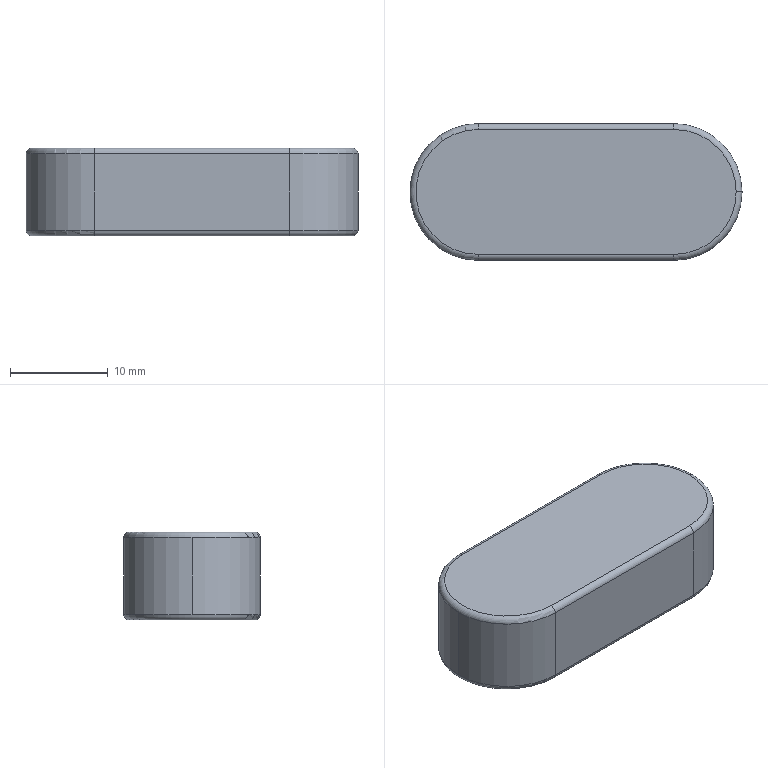Part | SolidWorks | features Extrusion 1, Fillet 1 | 1 solid | 17 faces | box 34 x 14 x 9 mm | volume 3893 mm3 | cylinder 7 | torus 6 | plane 4 | commonest cylinder face diameters 1.2 x4 14 x3
STEP:
#1=CARTESIAN_POINT('',(16.4,0.,0.));
#2=VERTEX_POINT('',#1);
#3=CARTESIAN_POINT('',(10.,-6.4,0.));
#4=VERTEX_POINT('',#3);
#5=CARTESIAN_POINT('',(10.,0.,0.));
#6=DIRECTION('',(0.,0.,-1.));
#7=DIRECTION('',(1.,0.,0.));
#8=AXIS2_PLACEMENT_3D('',#5,#6,#7);
#9=CIRCLE('',#8,6.4);
#10=EDGE_CURVE('',#2,#4,#9,.T.);
#11=ORIENTED_EDGE('',*,*,#10,.F.);
#12=CARTESIAN_POINT('',(17.,0.,0.6));
#13=VERTEX_POINT('',#12);
#14=CARTESIAN_POINT('',(16.4,0.,0.6));
#15=DIRECTION('',(0.,-1.,0.));
#16=DIRECTION('',(0.,0.,-1.));
#17=AXIS2_PLACEMENT_3D('',#14,#15,#16);
#18=CIRCLE('',#17,0.6);
#19=EDGE_CURVE('',#2,#13,#18,.T.);
#20=ORIENTED_EDGE('',*,*,#19,.T.);
#21=CARTESIAN_POINT('',(10.,-7.,0.6));
#22=VERTEX_POINT('',#21);
#23=CARTESIAN_POINT('',(10.,0.,0.6));
#24=DIRECTION('',(0.,0.,1.));
#25=DIRECTION('',(1.,0.,0.));
#26=AXIS2_PLACEMENT_3D('',#23,#24,#25);
#27=CIRCLE('',#26,7.);
#28=EDGE_CURVE('',#22,#13,#27,.T.);
#29=ORIENTED_EDGE('',*,*,#28,.F.);
#30=CARTESIAN_POINT('',(10.,-6.4,0.6));
#31=DIRECTION('',(1.,0.,0.));
#32=DIRECTION('',(0.,0.,-1.));
#33=AXIS2_PLACEMENT_3D('',#30,#31,#32);
#34=CIRCLE('',#33,0.6);
#35=EDGE_CURVE('',#22,#4,#34,.T.);
#36=ORIENTED_EDGE('',*,*,#35,.T.);
#37=EDGE_LOOP('',(#11,#20,#29,#36));
#38=FACE_OUTER_BOUND('',#37,.T.);
#39=CARTESIAN_POINT('',(10.,0.,0.6));
#40=DIRECTION('',(0.,0.,1.));
#41=DIRECTION('',(1.,0.,0.));
#42=AXIS2_PLACEMENT_3D('',#39,#40,#41);
#43=TOROIDAL_SURFACE('',#42,6.4,0.6);
#44=ADVANCED_FACE('',(#38),#43,.T.);
#45=CARTESIAN_POINT('',(17.,0.,8.4));
#46=VERTEX_POINT('',#45);
#47=CARTESIAN_POINT('',(10.,-7.,8.4));
#48=VERTEX_POINT('',#47);
#49=CARTESIAN_POINT('',(10.,0.,8.4));
#50=DIRECTION('',(0.,0.,-1.));
#51=DIRECTION('',(1.,0.,0.));
#52=AXIS2_PLACEMENT_3D('',#49,#50,#51);
#53=CIRCLE('',#52,7.);
#54=EDGE_CURVE('',#46,#48,#53,.T.);
#55=ORIENTED_EDGE('',*,*,#54,.F.);
#56=CARTESIAN_POINT('',(16.4,0.,9.));
#57=VERTEX_POINT('',#56);
#58=CARTESIAN_POINT('',(16.4,0.,8.4));
#59=DIRECTION('',(0.,-1.,0.));
#60=DIRECTION('',(0.,0.,-1.));
#61=AXIS2_PLACEMENT_3D('',#58,#59,#60);
#62=CIRCLE('',#61,0.6);
#63=EDGE_CURVE('',#46,#57,#62,.T.);
#64=ORIENTED_EDGE('',*,*,#63,.T.);
#65=CARTESIAN_POINT('',(10.,-6.4,9.));
#66=VERTEX_POINT('',#65);
#67=CARTESIAN_POINT('',(10.,0.,9.));
#68=DIRECTION('',(0.,0.,1.));
#69=DIRECTION('',(1.,0.,0.));
#70=AXIS2_PLACEMENT_3D('',#67,#68,#69);
#71=CIRCLE('',#70,6.4);
#72=EDGE_CURVE('',#66,#57,#71,.T.);
#73=ORIENTED_EDGE('',*,*,#72,.F.);
#74=CARTESIAN_POINT('',(10.,-6.4,8.4));
#75=DIRECTION('',(1.,0.,0.));
#76=DIRECTION('',(0.,0.,-1.));
#77=AXIS2_PLACEMENT_3D('',#74,#75,#76);
#78=CIRCLE('',#77,0.6);
#79=EDGE_CURVE('',#66,#48,#78,.T.);
#80=ORIENTED_EDGE('',*,*,#79,.T.);
#81=EDGE_LOOP('',(#55,#64,#73,#80));
#82=FACE_OUTER_BOUND('',#81,.T.);
#83=CARTESIAN_POINT('',(10.,0.,8.4));
#84=DIRECTION('',(0.,0.,1.));
#85=DIRECTION('',(1.,0.,0.));
#86=AXIS2_PLACEMENT_3D('',#83,#84,#85);
#87=TOROIDAL_SURFACE('',#86,6.4,0.6);
#88=ADVANCED_FACE('',(#82),#87,.T.);
#89=CARTESIAN_POINT('',(-10.,-7.,8.4));
#90=VERTEX_POINT('',#89);
#91=CARTESIAN_POINT('',(-17.,0.,8.4));
#92=VERTEX_POINT('',#91);
#93=CARTESIAN_POINT('',(-10.,0.,8.4));
#94=DIRECTION('',(0.,0.,-1.));
#95=DIRECTION('',(1.,0.,0.));
#96=AXIS2_PLACEMENT_3D('',#93,#94,#95);
#97=CIRCLE('',#96,7.);
#98=EDGE_CURVE('',#90,#92,#97,.T.);
#99=ORIENTED_EDGE('',*,*,#98,.T.);
#100=CARTESIAN_POINT('',(-17.,0.,0.6));
#101=VERTEX_POINT('',#100);
#102=CARTESIAN_POINT('',(-17.,0.,9.));
#103=DIRECTION('',(0.,0.,-1.));
#104=VECTOR('',#103,1000.);
#105=LINE('',#102,#104);
#106=EDGE_CURVE('',#92,#101,#105,.T.);
#107=ORIENTED_EDGE('',*,*,#106,.T.);
#108=CARTESIAN_POINT('',(-10.,-7.,0.6));
#109=VERTEX_POINT('',#108);
#110=CARTESIAN_POINT('',(-10.,0.,0.6));
#111=DIRECTION('',(0.,0.,1.));
#112=DIRECTION('',(1.,0.,0.));
#113=AXIS2_PLACEMENT_3D('',#110,#111,#112);
#114=CIRCLE('',#113,7.);
#115=EDGE_CURVE('',#101,#109,#114,.T.);
#116=ORIENTED_EDGE('',*,*,#115,.T.);
#117=CARTESIAN_POINT('',(-10.,-7.,9.));
#118=DIRECTION('',(0.,0.,-1.));
#119=VECTOR('',#118,1000.);
#120=LINE('',#117,#119);
#121=EDGE_CURVE('',#90,#109,#120,.T.);
#122=ORIENTED_EDGE('',*,*,#121,.F.);
#123=EDGE_LOOP('',(#99,#107,#116,#122));
#124=FACE_OUTER_BOUND('',#123,.T.);
#125=CARTESIAN_POINT('',(-10.,0.,9.));
#126=DIRECTION('',(0.,0.,-1.));
#127=DIRECTION('',(-1.,0.,0.));
#128=AXIS2_PLACEMENT_3D('',#125,#126,#127);
#129=CYLINDRICAL_SURFACE('',#128,7.);
#130=ADVANCED_FACE('',(#124),#129,.T.);
#131=ORIENTED_EDGE('',*,*,#106,.F.);
#132=CARTESIAN_POINT('',(-10.,7.,8.4));
#133=VERTEX_POINT('',#132);
#134=CARTESIAN_POINT('',(-10.,0.,8.4));
#135=DIRECTION('',(0.,0.,-1.));
#136=DIRECTION('',(1.,0.,0.));
#137=AXIS2_PLACEMENT_3D('',#134,#135,#136);
#138=CIRCLE('',#137,7.);
#139=EDGE_CURVE('',#92,#133,#138,.T.);
#140=ORIENTED_EDGE('',*,*,#139,.T.);
#141=CARTESIAN_POINT('',(-10.,7.,0.6));
#142=VERTEX_POINT('',#141);
#143=CARTESIAN_POINT('',(-10.,7.,9.));
#144=DIRECTION('',(0.,0.,-1.));
#145=VECTOR('',#144,1000.);
#146=LINE('',#143,#145);
#147=EDGE_CURVE('',#133,#142,#146,.T.);
#148=ORIENTED_EDGE('',*,*,#147,.T.);
#149=CARTESIAN_POINT('',(-10.,0.,0.6));
#150=DIRECTION('',(0.,0.,1.));
#151=DIRECTION('',(1.,0.,0.));
#152=AXIS2_PLACEMENT_3D('',#149,#150,#151);
#153=CIRCLE('',#152,7.);
#154=EDGE_CURVE('',#142,#101,#153,.T.);
#155=ORIENTED_EDGE('',*,*,#154,.T.);
#156=EDGE_LOOP('',(#131,#140,#148,#155));
#157=FACE_OUTER_BOUND('',#156,.T.);
#158=CARTESIAN_POINT('',(-10.,0.,9.));
#159=DIRECTION('',(0.,0.,-1.));
#160=DIRECTION('',(-1.,0.,0.));
#161=AXIS2_PLACEMENT_3D('',#158,#159,#160);
#162=CYLINDRICAL_SURFACE('',#161,7.);
#163=ADVANCED_FACE('',(#157),#162,.T.);
#164=CARTESIAN_POINT('',(10.,-7.,9.));
#165=DIRECTION('',(0.,0.,-1.));
#166=VECTOR('',#165,1000.);
#167=LINE('',#164,#166);
#168=EDGE_CURVE('',#48,#22,#167,.T.);
#169=ORIENTED_EDGE('',*,*,#168,.F.);
#170=CARTESIAN_POINT('',(-10.,-7.,8.4));
#171=DIRECTION('',(-1.,0.,0.));
#172=VECTOR('',#171,1000.);
#173=LINE('',#170,#172);
#174=EDGE_CURVE('',#48,#90,#173,.T.);
#175=ORIENTED_EDGE('',*,*,#174,.T.);
#176=ORIENTED_EDGE('',*,*,#121,.T.);
#177=CARTESIAN_POINT('',(-10.,-7.,0.6));
#178=DIRECTION('',(1.,0.,0.));
#179=VECTOR('',#178,1000.);
#180=LINE('',#177,#179);
#181=EDGE_CURVE('',#109,#22,#180,.T.);
#182=ORIENTED_EDGE('',*,*,#181,.T.);
#183=EDGE_LOOP('',(#169,#175,#176,#182));
#184=FACE_OUTER_BOUND('',#183,.T.);
#185=CARTESIAN_POINT('',(-10.,-7.,9.));
#186=DIRECTION('',(0.,1.,0.));
#187=DIRECTION('',(-1.,0.,0.));
#188=AXIS2_PLACEMENT_3D('',#185,#186,#187);
#189=PLANE('',#188);
#190=ADVANCED_FACE('',(#184),#189,.F.);
#191=CARTESIAN_POINT('',(10.,7.,8.4));
#192=VERTEX_POINT('',#191);
#193=CARTESIAN_POINT('',(10.,7.,0.6));
#194=VERTEX_POINT('',#193);
#195=CARTESIAN_POINT('',(10.,7.,9.));
#196=DIRECTION('',(0.,0.,-1.));
#197=VECTOR('',#196,1000.);
#198=LINE('',#195,#197);
#199=EDGE_CURVE('',#192,#194,#198,.T.);
#200=ORIENTED_EDGE('',*,*,#199,.F.);
#201=CARTESIAN_POINT('',(10.,0.,8.4));
#202=DIRECTION('',(0.,0.,-1.));
#203=DIRECTION('',(1.,0.,0.));
#204=AXIS2_PLACEMENT_3D('',#201,#202,#203);
#205=CIRCLE('',#204,7.);
#206=EDGE_CURVE('',#192,#46,#205,.T.);
#207=ORIENTED_EDGE('',*,*,#206,.T.);
#208=ORIENTED_EDGE('',*,*,#54,.T.);
#209=ORIENTED_EDGE('',*,*,#168,.T.);
#210=ORIENTED_EDGE('',*,*,#28,.T.);
#211=CARTESIAN_POINT('',(10.,0.,0.6));
#212=DIRECTION('',(0.,0.,1.));
#213=DIRECTION('',(1.,0.,0.));
#214=AXIS2_PLACEMENT_3D('',#211,#212,#213);
#215=CIRCLE('',#214,7.);
#216=EDGE_CURVE('',#13,#194,#215,.T.);
#217=ORIENTED_EDGE('',*,*,#216,.T.);
#218=EDGE_LOOP('',(#200,#207,#208,#209,#210,#217));
#219=FACE_OUTER_BOUND('',#218,.T.);
#220=CARTESIAN_POINT('',(10.,0.,9.));
#221=DIRECTION('',(0.,0.,-1.));
#222=DIRECTION('',(-1.,0.,0.));
#223=AXIS2_PLACEMENT_3D('',#220,#221,#222);
#224=CYLINDRICAL_SURFACE('',#223,7.);
#225=ADVANCED_FACE('',(#219),#224,.T.);
#226=ORIENTED_EDGE('',*,*,#147,.F.);
#227=CARTESIAN_POINT('',(10.,7.,8.4));
#228=DIRECTION('',(1.,0.,0.));
#229=VECTOR('',#228,1000.);
#230=LINE('',#227,#229);
#231=EDGE_CURVE('',#133,#192,#230,.T.);
#232=ORIENTED_EDGE('',*,*,#231,.T.);
#233=ORIENTED_EDGE('',*,*,#199,.T.);
#234=CARTESIAN_POINT('',(-10.,7.,0.6));
#235=DIRECTION('',(-1.,0.,0.));
#236=VECTOR('',#235,1000.);
#237=LINE('',#234,#236);
#238=EDGE_CURVE('',#194,#142,#237,.T.);
#239=ORIENTED_EDGE('',*,*,#238,.T.);
#240=EDGE_LOOP('',(#226,#232,#233,#239));
#241=FACE_OUTER_BOUND('',#240,.T.);
#242=CARTESIAN_POINT('',(-10.,7.,9.));
#243=DIRECTION('',(0.,-1.,0.));
#244=DIRECTION('',(1.,0.,0.));
#245=AXIS2_PLACEMENT_3D('',#242,#243,#244);
#246=PLANE('',#245);
#247=ADVANCED_FACE('',(#241),#246,.F.);
#248=CARTESIAN_POINT('',(-10.,-6.4,9.));
#249=VERTEX_POINT('',#248);
#250=CARTESIAN_POINT('',(10.,-6.4,9.));
#251=DIRECTION('',(1.,0.,0.));
#252=VECTOR('',#251,1000.);
#253=LINE('',#250,#252);
#254=EDGE_CURVE('',#249,#66,#253,.T.);
#255=ORIENTED_EDGE('',*,*,#254,.T.);
#256=ORIENTED_EDGE('',*,*,#72,.T.);
#257=CARTESIAN_POINT('',(10.,6.4,9.));
#258=VERTEX_POINT('',#257);
#259=CARTESIAN_POINT('',(10.,0.,9.));
#260=DIRECTION('',(0.,0.,1.));
#261=DIRECTION('',(1.,0.,0.));
#262=AXIS2_PLACEMENT_3D('',#259,#260,#261);
#263=CIRCLE('',#262,6.4);
#264=EDGE_CURVE('',#57,#258,#263,.T.);
#265=ORIENTED_EDGE('',*,*,#264,.T.);
#266=CARTESIAN_POINT('',(-10.,6.4,9.));
#267=VERTEX_POINT('',#266);
#268=CARTESIAN_POINT('',(-10.,6.4,9.));
#269=DIRECTION('',(-1.,0.,0.));
#270=VECTOR('',#269,1000.);
#271=LINE('',#268,#270);
#272=EDGE_CURVE('',#258,#267,#271,.T.);
#273=ORIENTED_EDGE('',*,*,#272,.T.);
#274=CARTESIAN_POINT('',(-10.,0.,9.));
#275=DIRECTION('',(0.,0.,1.));
#276=DIRECTION('',(1.,0.,0.));
#277=AXIS2_PLACEMENT_3D('',#274,#275,#276);
#278=CIRCLE('',#277,6.4);
#279=EDGE_CURVE('',#267,#249,#278,.T.);
#280=ORIENTED_EDGE('',*,*,#279,.T.);
#281=EDGE_LOOP('',(#255,#256,#265,#273,#280));
#282=FACE_OUTER_BOUND('',#281,.T.);
#283=CARTESIAN_POINT('',(-10.,0.,9.));
#284=DIRECTION('',(0.,0.,1.));
#285=DIRECTION('',(1.,0.,0.));
#286=AXIS2_PLACEMENT_3D('',#283,#284,#285);
#287=PLANE('',#286);
#288=ADVANCED_FACE('',(#282),#287,.T.);
#289=CARTESIAN_POINT('',(-10.,6.4,0.));
#290=VERTEX_POINT('',#289);
#291=CARTESIAN_POINT('',(10.,6.4,0.));
#292=VERTEX_POINT('',#291);
#293=CARTESIAN_POINT('',(-10.,6.4,0.));
#294=DIRECTION('',(1.,0.,0.));
#295=VECTOR('',#294,1000.);
#296=LINE('',#293,#295);
#297=EDGE_CURVE('',#290,#292,#296,.T.);
#298=ORIENTED_EDGE('',*,*,#297,.T.);
#299=CARTESIAN_POINT('',(10.,0.,0.));
#300=DIRECTION('',(0.,0.,-1.));
#301=DIRECTION('',(1.,0.,0.));
#302=AXIS2_PLACEMENT_3D('',#299,#300,#301);
#303=CIRCLE('',#302,6.4);
#304=EDGE_CURVE('',#292,#2,#303,.T.);
#305=ORIENTED_EDGE('',*,*,#304,.T.);
#306=ORIENTED_EDGE('',*,*,#10,.T.);
#307=CARTESIAN_POINT('',(-10.,-6.4,0.));
#308=VERTEX_POINT('',#307);
#309=CARTESIAN_POINT('',(-10.,-6.4,0.));
#310=DIRECTION('',(-1.,0.,0.));
#311=VECTOR('',#310,1000.);
#312=LINE('',#309,#311);
#313=EDGE_CURVE('',#4,#308,#312,.T.);
#314=ORIENTED_EDGE('',*,*,#313,.T.);
#315=CARTESIAN_POINT('',(-10.,0.,0.));
#316=DIRECTION('',(0.,0.,-1.));
#317=DIRECTION('',(1.,0.,0.));
#318=AXIS2_PLACEMENT_3D('',#315,#316,#317);
#319=CIRCLE('',#318,6.4);
#320=EDGE_CURVE('',#308,#290,#319,.T.);
#321=ORIENTED_EDGE('',*,*,#320,.T.);
#322=EDGE_LOOP('',(#298,#305,#306,#314,#321));
#323=FACE_OUTER_BOUND('',#322,.T.);
#324=CARTESIAN_POINT('',(-10.,0.,0.));
#325=DIRECTION('',(0.,0.,1.));
#326=DIRECTION('',(1.,0.,0.));
#327=AXIS2_PLACEMENT_3D('',#324,#325,#326);
#328=PLANE('',#327);
#329=ADVANCED_FACE('',(#323),#328,.F.);
#330=CARTESIAN_POINT('',(-10.,6.4,8.4));
#331=DIRECTION('',(1.,0.,0.));
#332=DIRECTION('',(0.,0.,-1.));
#333=AXIS2_PLACEMENT_3D('',#330,#331,#332);
#334=CIRCLE('',#333,0.6);
#335=EDGE_CURVE('',#133,#267,#334,.T.);
#336=ORIENTED_EDGE('',*,*,#335,.F.);
#337=ORIENTED_EDGE('',*,*,#139,.F.);
#338=ORIENTED_EDGE('',*,*,#98,.F.);
#339=CARTESIAN_POINT('',(-10.,-6.4,8.4));
#340=DIRECTION('',(1.,0.,0.));
#341=DIRECTION('',(0.,0.,-1.));
#342=AXIS2_PLACEMENT_3D('',#339,#340,#341);
#343=CIRCLE('',#342,0.6);
#344=EDGE_CURVE('',#249,#90,#343,.T.);
#345=ORIENTED_EDGE('',*,*,#344,.F.);
#346=ORIENTED_EDGE('',*,*,#279,.F.);
#347=EDGE_LOOP('',(#336,#337,#338,#345,#346));
#348=FACE_OUTER_BOUND('',#347,.T.);
#349=CARTESIAN_POINT('',(-10.,0.,8.4));
#350=DIRECTION('',(0.,0.,1.));
#351=DIRECTION('',(1.,0.,0.));
#352=AXIS2_PLACEMENT_3D('',#349,#350,#351);
#353=TOROIDAL_SURFACE('',#352,6.4,0.6);
#354=ADVANCED_FACE('',(#348),#353,.T.);
#355=ORIENTED_EDGE('',*,*,#344,.T.);
#356=ORIENTED_EDGE('',*,*,#174,.F.);
#357=ORIENTED_EDGE('',*,*,#79,.F.);
#358=ORIENTED_EDGE('',*,*,#254,.F.);
#359=EDGE_LOOP('',(#355,#356,#357,#358));
#360=FACE_OUTER_BOUND('',#359,.T.);
#361=CARTESIAN_POINT('',(-10.,-6.4,8.4));
#362=DIRECTION('',(-1.,0.,0.));
#363=DIRECTION('',(0.,-1.,0.));
#364=AXIS2_PLACEMENT_3D('',#361,#362,#363);
#365=CYLINDRICAL_SURFACE('',#364,0.6);
#366=ADVANCED_FACE('',(#360),#365,.T.);
#367=ORIENTED_EDGE('',*,*,#335,.T.);
#368=ORIENTED_EDGE('',*,*,#272,.F.);
#369=CARTESIAN_POINT('',(10.,6.4,8.4));
#370=DIRECTION('',(1.,0.,0.));
#371=DIRECTION('',(0.,0.,-1.));
#372=AXIS2_PLACEMENT_3D('',#369,#370,#371);
#373=CIRCLE('',#372,0.6);
#374=EDGE_CURVE('',#192,#258,#373,.T.);
#375=ORIENTED_EDGE('',*,*,#374,.F.);
#376=ORIENTED_EDGE('',*,*,#231,.F.);
#377=EDGE_LOOP('',(#367,#368,#375,#376));
#378=FACE_OUTER_BOUND('',#377,.T.);
#379=CARTESIAN_POINT('',(-10.,6.4,8.4));
#380=DIRECTION('',(1.,0.,0.));
#381=DIRECTION('',(0.,1.,0.));
#382=AXIS2_PLACEMENT_3D('',#379,#380,#381);
#383=CYLINDRICAL_SURFACE('',#382,0.6);
#384=ADVANCED_FACE('',(#378),#383,.T.);
#385=ORIENTED_EDGE('',*,*,#63,.F.);
#386=ORIENTED_EDGE('',*,*,#206,.F.);
#387=ORIENTED_EDGE('',*,*,#374,.T.);
#388=ORIENTED_EDGE('',*,*,#264,.F.);
#389=EDGE_LOOP('',(#385,#386,#387,#388));
#390=FACE_OUTER_BOUND('',#389,.T.);
#391=CARTESIAN_POINT('',(10.,0.,8.4));
#392=DIRECTION('',(0.,0.,1.));
#393=DIRECTION('',(1.,0.,0.));
#394=AXIS2_PLACEMENT_3D('',#391,#392,#393);
#395=TOROIDAL_SURFACE('',#394,6.4,0.6);
#396=ADVANCED_FACE('',(#390),#395,.T.);
#397=CARTESIAN_POINT('',(-10.,6.4,0.6));
#398=DIRECTION('',(1.,0.,0.));
#399=DIRECTION('',(0.,0.,-1.));
#400=AXIS2_PLACEMENT_3D('',#397,#398,#399);
#401=CIRCLE('',#400,0.6);
#402=EDGE_CURVE('',#290,#142,#401,.T.);
#403=ORIENTED_EDGE('',*,*,#402,.F.);
#404=ORIENTED_EDGE('',*,*,#320,.F.);
#405=CARTESIAN_POINT('',(-10.,-6.4,0.6));
#406=DIRECTION('',(1.,0.,0.));
#407=DIRECTION('',(0.,0.,-1.));
#408=AXIS2_PLACEMENT_3D('',#405,#406,#407);
#409=CIRCLE('',#408,0.6);
#410=EDGE_CURVE('',#109,#308,#409,.T.);
#411=ORIENTED_EDGE('',*,*,#410,.F.);
#412=ORIENTED_EDGE('',*,*,#115,.F.);
#413=ORIENTED_EDGE('',*,*,#154,.F.);
#414=EDGE_LOOP('',(#403,#404,#411,#412,#413));
#415=FACE_OUTER_BOUND('',#414,.T.);
#416=CARTESIAN_POINT('',(-10.,0.,0.6));
#417=DIRECTION('',(0.,0.,1.));
#418=DIRECTION('',(1.,0.,0.));
#419=AXIS2_PLACEMENT_3D('',#416,#417,#418);
#420=TOROIDAL_SURFACE('',#419,6.4,0.6);
#421=ADVANCED_FACE('',(#415),#420,.T.);
#422=ORIENTED_EDGE('',*,*,#410,.T.);
#423=ORIENTED_EDGE('',*,*,#313,.F.);
#424=ORIENTED_EDGE('',*,*,#35,.F.);
#425=ORIENTED_EDGE('',*,*,#181,.F.);
#426=EDGE_LOOP('',(#422,#423,#424,#425));
#427=FACE_OUTER_BOUND('',#426,.T.);
#428=CARTESIAN_POINT('',(-10.,-6.4,0.6));
#429=DIRECTION('',(1.,0.,0.));
#430=DIRECTION('',(0.,1.,0.));
#431=AXIS2_PLACEMENT_3D('',#428,#429,#430);
#432=CYLINDRICAL_SURFACE('',#431,0.6);
#433=ADVANCED_FACE('',(#427),#432,.T.);
#434=ORIENTED_EDGE('',*,*,#402,.T.);
#435=ORIENTED_EDGE('',*,*,#238,.F.);
#436=CARTESIAN_POINT('',(10.,6.4,0.6));
#437=DIRECTION('',(1.,0.,0.));
#438=DIRECTION('',(0.,0.,-1.));
#439=AXIS2_PLACEMENT_3D('',#436,#437,#438);
#440=CIRCLE('',#439,0.6);
#441=EDGE_CURVE('',#292,#194,#440,.T.);
#442=ORIENTED_EDGE('',*,*,#441,.F.);
#443=ORIENTED_EDGE('',*,*,#297,.F.);
#444=EDGE_LOOP('',(#434,#435,#442,#443));
#445=FACE_OUTER_BOUND('',#444,.T.);
#446=CARTESIAN_POINT('',(-10.,6.4,0.6));
#447=DIRECTION('',(-1.,0.,0.));
#448=DIRECTION('',(0.,-1.,0.));
#449=AXIS2_PLACEMENT_3D('',#446,#447,#448);
#450=CYLINDRICAL_SURFACE('',#449,0.6);
#451=ADVANCED_FACE('',(#445),#450,.T.);
#452=ORIENTED_EDGE('',*,*,#19,.F.);
#453=ORIENTED_EDGE('',*,*,#304,.F.);
#454=ORIENTED_EDGE('',*,*,#441,.T.);
#455=ORIENTED_EDGE('',*,*,#216,.F.);
#456=EDGE_LOOP('',(#452,#453,#454,#455));
#457=FACE_OUTER_BOUND('',#456,.T.);
#458=CARTESIAN_POINT('',(10.,0.,0.6));
#459=DIRECTION('',(0.,0.,1.));
#460=DIRECTION('',(1.,0.,0.));
#461=AXIS2_PLACEMENT_3D('',#458,#459,#460);
#462=TOROIDAL_SURFACE('',#461,6.4,0.6);
#463=ADVANCED_FACE('',(#457),#462,.T.);
#464=CLOSED_SHELL('',(#44,#88,#130,#163,#190,#225,#247,#288,#329,#354,#366,#384,#396,#421,#433,#451,#463));
#465=MANIFOLD_SOLID_BREP('',#464);
#466=CARTESIAN_POINT('',(0.,0.,0.));
#467=DIRECTION('',(0.,0.,1.));
#468=DIRECTION('',(1.,0.,0.));
#469=AXIS2_PLACEMENT_3D('',#466,#467,#468);
#470=(LENGTH_UNIT()NAMED_UNIT(*)SI_UNIT(.MILLI.,.METRE.));
#471=UNCERTAINTY_MEASURE_WITH_UNIT(LENGTH_MEASURE(0.00001),#470,'','');
#472=(NAMED_UNIT(*)PLANE_ANGLE_UNIT()SI_UNIT($,.RADIAN.));
#473=(NAMED_UNIT(*)SI_UNIT($,.STERADIAN.)SOLID_ANGLE_UNIT());
#474=(GEOMETRIC_REPRESENTATION_CONTEXT(3)GLOBAL_UNCERTAINTY_ASSIGNED_CONTEXT((#471))GLOBAL_UNIT_ASSIGNED_CONTEXT((#470,#472,#473))REPRESENTATION_CONTEXT('',''));
#475=ADVANCED_BREP_SHAPE_REPRESENTATION('',(#465,#469),#474);